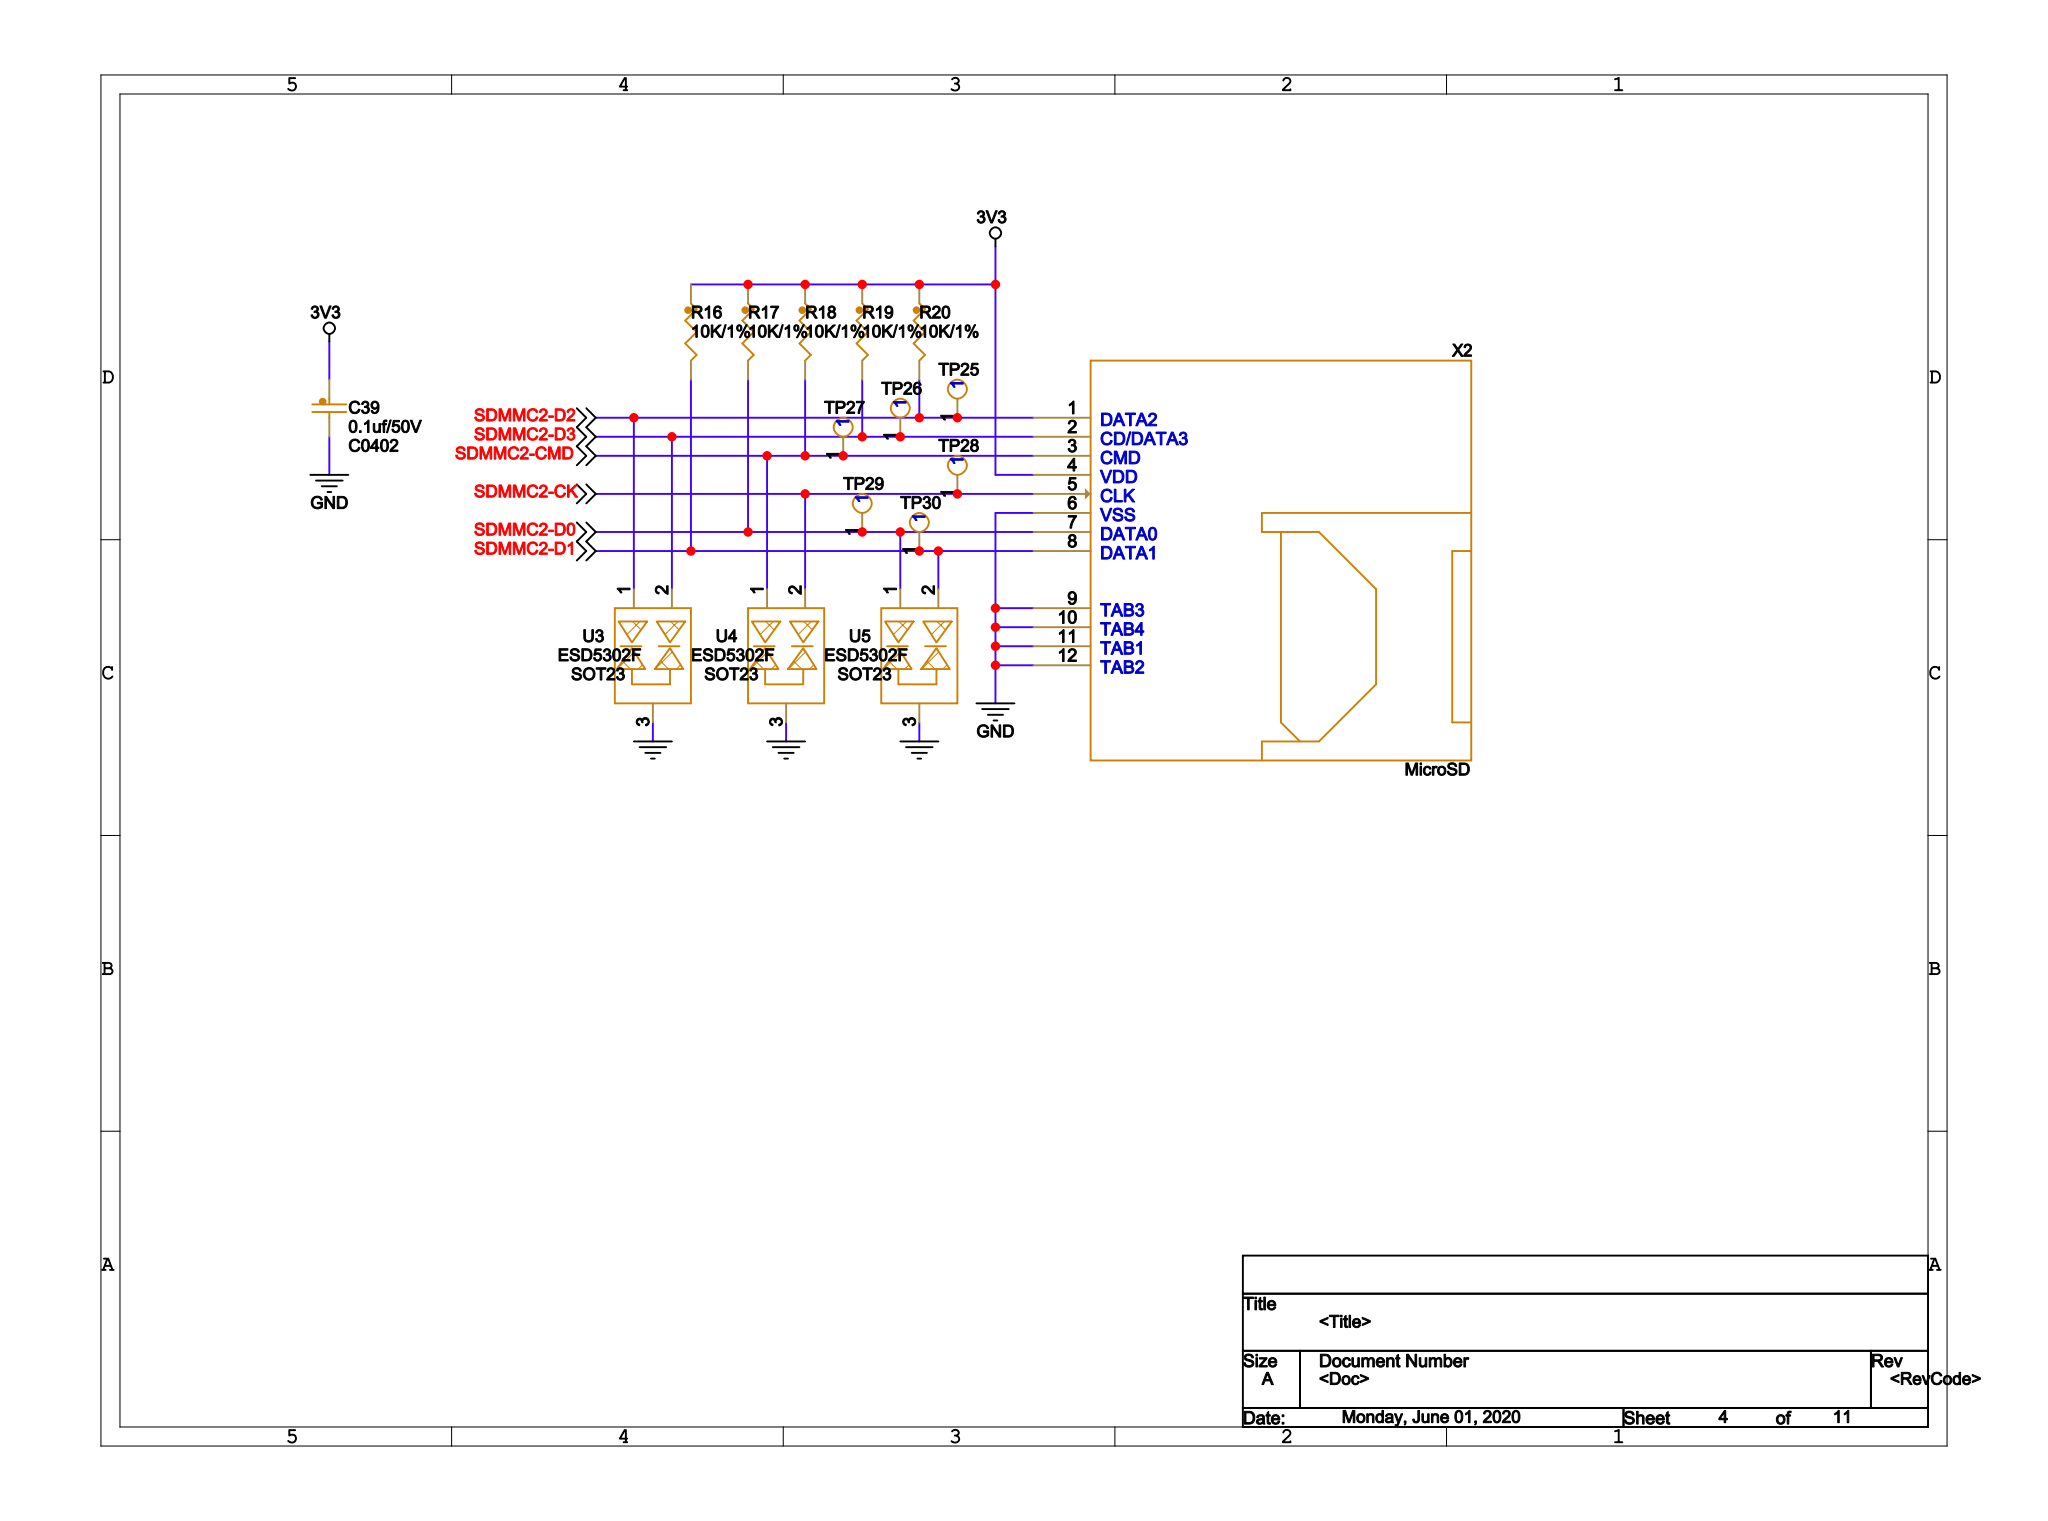Circuit board | Cadence Allegro | 792 parts | 400 nets | one sheet of the schematic
Parts on this sheet (reference | value | footprint):
C39 | 0.1uf/50V | C0402
R16 | 10K/1% | 0402
R17 | 10K/1% | 0402
R18 | 10K/1% | 0402
R19 | 10K/1% | 0402
R20 | 10K/1% | 0402
TP25 | TESTPOINT | TESTPOINT-33MIL
TP26 | TESTPOINT | TESTPOINT-33MIL
TP27 | TESTPOINT | TESTPOINT-33MIL
TP28 | TESTPOINT | TESTPOINT-33MIL
TP29 | TESTPOINT | TESTPOINT-33MIL
TP30 | TESTPOINT | TESTPOINT-33MIL
U3 | ESD5302F | SOT23
U4 | ESD5302F | SOT23
U5 | ESD5302F | SOT23
X2 | MicroSD | TFCARD-TF-02A
Nets of these parts (net: part-pin ...):
3V3: C39-1 R16-1 R17-1 R18-1 R19-1 R20-1 X2-4
GND: C39-2 U3-3 U4-3 U5-3 X2-6 X2-9 X2-10 X2-11 X2-12
SDMMC2-D2: R20-2 TP25-1 U3-1 X2-1
SDMMC2-D3: R19-2 TP26-1 U3-2 X2-2
SDMMC2-CMD: R18-2 TP27-1 U4-1 X2-3
SDMMC2-CK: TP28-1 U4-2 X2-5
SDMMC2-D0: R17-2 TP29-1 U5-1 X2-7
SDMMC2-D1: R16-2 TP30-1 U5-2 X2-8